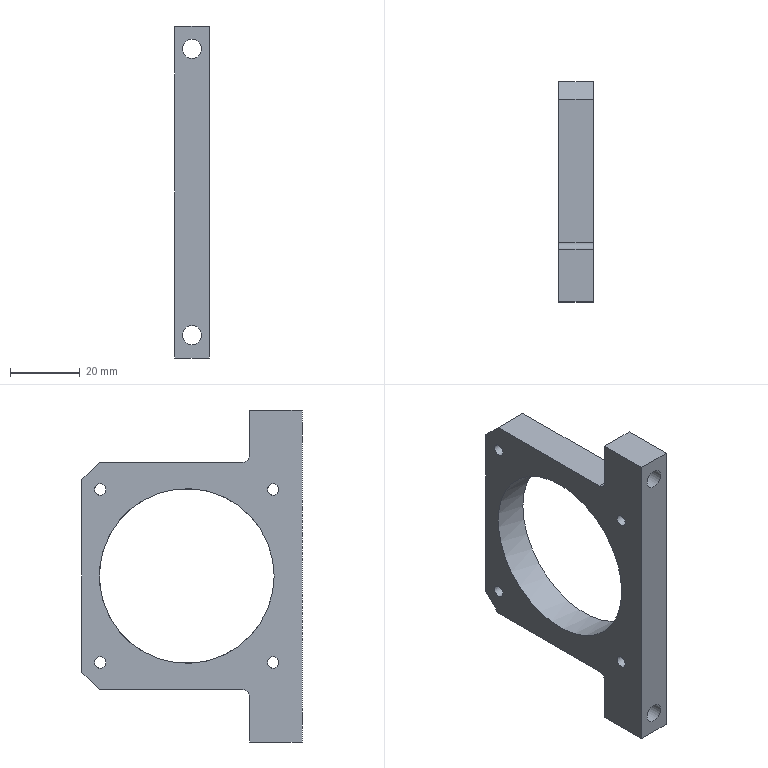Part | NX | 1 solid | 21 faces | box 10 x 63 x 95 mm | volume 24527 mm3 | plane 12 | cylinder 9 | commonest cylinder face diameters 3.3 x4 4 x2 5.5 x2 50 x1
STEP:
#1=CARTESIAN_POINT('',(-10.,42.749,-23.099));
#2=VERTEX_POINT('',#1);
#3=CARTESIAN_POINT('',(-10.,42.749,-24.749));
#4=DIRECTION('',(-1.,0.,0.));
#5=DIRECTION('',(0.,0.,1.));
#6=AXIS2_PLACEMENT_3D('',#3,#4,#5);
#7=CIRCLE('',#6,1.65);
#8=EDGE_CURVE('',#2,#2,#7,.T.);
#9=ORIENTED_EDGE('',*,*,#8,.F.);
#10=EDGE_LOOP('',(#9));
#11=FACE_BOUND('',#10,.T.);
#12=CARTESIAN_POINT('',(-10.,42.749,26.399));
#13=VERTEX_POINT('',#12);
#14=CARTESIAN_POINT('',(-10.,42.749,24.749));
#15=DIRECTION('',(-1.,0.,0.));
#16=DIRECTION('',(0.,0.,1.));
#17=AXIS2_PLACEMENT_3D('',#14,#15,#16);
#18=CIRCLE('',#17,1.65);
#19=EDGE_CURVE('',#13,#13,#18,.T.);
#20=ORIENTED_EDGE('',*,*,#19,.F.);
#21=EDGE_LOOP('',(#20));
#22=FACE_BOUND('',#21,.T.);
#23=CARTESIAN_POINT('',(-10.,-6.749,26.399));
#24=VERTEX_POINT('',#23);
#25=CARTESIAN_POINT('',(-10.,-6.749,24.749));
#26=DIRECTION('',(-1.,0.,0.));
#27=DIRECTION('',(0.,0.,1.));
#28=AXIS2_PLACEMENT_3D('',#25,#26,#27);
#29=CIRCLE('',#28,1.65);
#30=EDGE_CURVE('',#24,#24,#29,.T.);
#31=ORIENTED_EDGE('',*,*,#30,.F.);
#32=EDGE_LOOP('',(#31));
#33=FACE_BOUND('',#32,.T.);
#34=CARTESIAN_POINT('',(-10.,-6.749,-23.099));
#35=VERTEX_POINT('',#34);
#36=CARTESIAN_POINT('',(-10.,-6.749,-24.749));
#37=DIRECTION('',(-1.,0.,0.));
#38=DIRECTION('',(0.,0.,1.));
#39=AXIS2_PLACEMENT_3D('',#36,#37,#38);
#40=CIRCLE('',#39,1.65);
#41=EDGE_CURVE('',#35,#35,#40,.T.);
#42=ORIENTED_EDGE('',*,*,#41,.F.);
#43=EDGE_LOOP('',(#42));
#44=FACE_BOUND('',#43,.T.);
#45=CARTESIAN_POINT('',(-10.,-7.,0.));
#46=VERTEX_POINT('',#45);
#47=CARTESIAN_POINT('',(-10.,18.,0.));
#48=DIRECTION('',(-1.,0.,0.));
#49=DIRECTION('',(0.,-1.,0.));
#50=AXIS2_PLACEMENT_3D('',#47,#48,#49);
#51=CIRCLE('',#50,25.);
#52=EDGE_CURVE('',#46,#46,#51,.T.);
#53=ORIENTED_EDGE('',*,*,#52,.F.);
#54=EDGE_LOOP('',(#53));
#55=FACE_BOUND('',#54,.T.);
#56=CARTESIAN_POINT('',(-10.,48.,27.5));
#57=VERTEX_POINT('',#56);
#58=CARTESIAN_POINT('',(-10.,48.,-27.5));
#59=VERTEX_POINT('',#58);
#60=CARTESIAN_POINT('',(-10.,48.,32.5));
#61=DIRECTION('',(0.,0.,-1.));
#62=VECTOR('',#61,1000.);
#63=LINE('',#60,#62);
#64=EDGE_CURVE('',#57,#59,#63,.T.);
#65=ORIENTED_EDGE('',*,*,#64,.T.);
#66=CARTESIAN_POINT('',(-10.,43.,-32.5));
#67=VERTEX_POINT('',#66);
#68=CARTESIAN_POINT('',(-10.,43.,-32.5));
#69=DIRECTION('',(0.,0.7071,0.7071));
#70=VECTOR('',#69,1000.);
#71=LINE('',#68,#70);
#72=EDGE_CURVE('',#59,#67,#71,.F.);
#73=ORIENTED_EDGE('',*,*,#72,.T.);
#74=CARTESIAN_POINT('',(-10.,2.,-32.5));
#75=VERTEX_POINT('',#74);
#76=CARTESIAN_POINT('',(-10.,48.,-32.5));
#77=DIRECTION('',(0.,-1.,0.));
#78=VECTOR('',#77,1000.);
#79=LINE('',#76,#78);
#80=EDGE_CURVE('',#67,#75,#79,.T.);
#81=ORIENTED_EDGE('',*,*,#80,.T.);
#82=CARTESIAN_POINT('',(-10.,0.,-34.5));
#83=VERTEX_POINT('',#82);
#84=CARTESIAN_POINT('',(-10.,2.,-34.5));
#85=DIRECTION('',(1.,0.,0.));
#86=DIRECTION('',(0.,1.,0.));
#87=AXIS2_PLACEMENT_3D('',#84,#85,#86);
#88=CIRCLE('',#87,2.);
#89=EDGE_CURVE('',#75,#83,#88,.T.);
#90=ORIENTED_EDGE('',*,*,#89,.T.);
#91=CARTESIAN_POINT('',(-10.,0.,-47.5));
#92=VERTEX_POINT('',#91);
#93=CARTESIAN_POINT('',(-10.,0.,-47.5));
#94=DIRECTION('',(0.,0.,-1.));
#95=VECTOR('',#94,1000.);
#96=LINE('',#93,#95);
#97=EDGE_CURVE('',#83,#92,#96,.T.);
#98=ORIENTED_EDGE('',*,*,#97,.T.);
#99=CARTESIAN_POINT('',(-10.,-15.,-47.5));
#100=VERTEX_POINT('',#99);
#101=CARTESIAN_POINT('',(-10.,-15.,-47.5));
#102=DIRECTION('',(0.,1.,0.));
#103=VECTOR('',#102,1000.);
#104=LINE('',#101,#103);
#105=EDGE_CURVE('',#100,#92,#104,.T.);
#106=ORIENTED_EDGE('',*,*,#105,.F.);
#107=CARTESIAN_POINT('',(-10.,-15.,47.5));
#108=VERTEX_POINT('',#107);
#109=CARTESIAN_POINT('',(-10.,-15.,-47.5));
#110=DIRECTION('',(0.,0.,-1.));
#111=VECTOR('',#110,1000.);
#112=LINE('',#109,#111);
#113=EDGE_CURVE('',#108,#100,#112,.T.);
#114=ORIENTED_EDGE('',*,*,#113,.F.);
#115=CARTESIAN_POINT('',(-10.,0.,47.5));
#116=VERTEX_POINT('',#115);
#117=CARTESIAN_POINT('',(-10.,-15.,47.5));
#118=DIRECTION('',(0.,1.,0.));
#119=VECTOR('',#118,1000.);
#120=LINE('',#117,#119);
#121=EDGE_CURVE('',#108,#116,#120,.T.);
#122=ORIENTED_EDGE('',*,*,#121,.T.);
#123=CARTESIAN_POINT('',(-10.,0.,34.5));
#124=VERTEX_POINT('',#123);
#125=CARTESIAN_POINT('',(-10.,0.,-47.5));
#126=DIRECTION('',(0.,0.,-1.));
#127=VECTOR('',#126,1000.);
#128=LINE('',#125,#127);
#129=EDGE_CURVE('',#116,#124,#128,.T.);
#130=ORIENTED_EDGE('',*,*,#129,.T.);
#131=CARTESIAN_POINT('',(-10.,2.,32.5));
#132=VERTEX_POINT('',#131);
#133=CARTESIAN_POINT('',(-10.,2.,34.5));
#134=DIRECTION('',(1.,0.,0.));
#135=DIRECTION('',(0.,1.,0.));
#136=AXIS2_PLACEMENT_3D('',#133,#134,#135);
#137=CIRCLE('',#136,2.);
#138=EDGE_CURVE('',#124,#132,#137,.T.);
#139=ORIENTED_EDGE('',*,*,#138,.T.);
#140=CARTESIAN_POINT('',(-10.,43.,32.5));
#141=VERTEX_POINT('',#140);
#142=CARTESIAN_POINT('',(-10.,48.,32.5));
#143=DIRECTION('',(0.,-1.,0.));
#144=VECTOR('',#143,1000.);
#145=LINE('',#142,#144);
#146=EDGE_CURVE('',#141,#132,#145,.T.);
#147=ORIENTED_EDGE('',*,*,#146,.F.);
#148=CARTESIAN_POINT('',(-10.,48.,27.5));
#149=DIRECTION('',(0.,0.7071,-0.7071));
#150=VECTOR('',#149,1000.);
#151=LINE('',#148,#150);
#152=EDGE_CURVE('',#141,#57,#151,.T.);
#153=ORIENTED_EDGE('',*,*,#152,.T.);
#154=EDGE_LOOP('',(#65,#73,#81,#90,#98,#106,#114,#122,#130,#139,#147,#153));
#155=FACE_BOUND('',#154,.T.);
#156=CARTESIAN_POINT('',(-10.,48.,32.5));
#157=DIRECTION('',(1.,0.,0.));
#158=DIRECTION('',(0.,1.,0.));
#159=AXIS2_PLACEMENT_3D('',#156,#157,#158);
#160=PLANE('',#159);
#161=ADVANCED_FACE('',(#11,#22,#33,#44,#55,#155),#160,.F.);
#162=CARTESIAN_POINT('',(0.,44.399,-24.749));
#163=VERTEX_POINT('',#162);
#164=CARTESIAN_POINT('',(0.,42.749,-24.749));
#165=DIRECTION('',(1.,0.,0.));
#166=DIRECTION('',(0.,1.,0.));
#167=AXIS2_PLACEMENT_3D('',#164,#165,#166);
#168=CIRCLE('',#167,1.65);
#169=EDGE_CURVE('',#163,#163,#168,.T.);
#170=ORIENTED_EDGE('',*,*,#169,.F.);
#171=EDGE_LOOP('',(#170));
#172=FACE_BOUND('',#171,.T.);
#173=CARTESIAN_POINT('',(0.,44.399,24.749));
#174=VERTEX_POINT('',#173);
#175=CARTESIAN_POINT('',(0.,42.749,24.749));
#176=DIRECTION('',(1.,0.,0.));
#177=DIRECTION('',(0.,1.,0.));
#178=AXIS2_PLACEMENT_3D('',#175,#176,#177);
#179=CIRCLE('',#178,1.65);
#180=EDGE_CURVE('',#174,#174,#179,.T.);
#181=ORIENTED_EDGE('',*,*,#180,.F.);
#182=EDGE_LOOP('',(#181));
#183=FACE_BOUND('',#182,.T.);
#184=CARTESIAN_POINT('',(0.,-5.099,24.749));
#185=VERTEX_POINT('',#184);
#186=CARTESIAN_POINT('',(0.,-6.749,24.749));
#187=DIRECTION('',(1.,0.,0.));
#188=DIRECTION('',(0.,1.,0.));
#189=AXIS2_PLACEMENT_3D('',#186,#187,#188);
#190=CIRCLE('',#189,1.65);
#191=EDGE_CURVE('',#185,#185,#190,.T.);
#192=ORIENTED_EDGE('',*,*,#191,.F.);
#193=EDGE_LOOP('',(#192));
#194=FACE_BOUND('',#193,.T.);
#195=CARTESIAN_POINT('',(0.,-5.099,-24.749));
#196=VERTEX_POINT('',#195);
#197=CARTESIAN_POINT('',(0.,-6.749,-24.749));
#198=DIRECTION('',(1.,0.,0.));
#199=DIRECTION('',(0.,1.,0.));
#200=AXIS2_PLACEMENT_3D('',#197,#198,#199);
#201=CIRCLE('',#200,1.65);
#202=EDGE_CURVE('',#196,#196,#201,.T.);
#203=ORIENTED_EDGE('',*,*,#202,.F.);
#204=EDGE_LOOP('',(#203));
#205=FACE_BOUND('',#204,.T.);
#206=CARTESIAN_POINT('',(0.,43.,0.));
#207=VERTEX_POINT('',#206);
#208=CARTESIAN_POINT('',(0.,18.,0.));
#209=DIRECTION('',(1.,0.,0.));
#210=DIRECTION('',(0.,1.,0.));
#211=AXIS2_PLACEMENT_3D('',#208,#209,#210);
#212=CIRCLE('',#211,25.);
#213=EDGE_CURVE('',#207,#207,#212,.T.);
#214=ORIENTED_EDGE('',*,*,#213,.F.);
#215=EDGE_LOOP('',(#214));
#216=FACE_BOUND('',#215,.T.);
#217=CARTESIAN_POINT('',(0.,43.,-32.5));
#218=VERTEX_POINT('',#217);
#219=CARTESIAN_POINT('',(0.,2.,-32.5));
#220=VERTEX_POINT('',#219);
#221=CARTESIAN_POINT('',(0.,48.,-32.5));
#222=DIRECTION('',(0.,-1.,0.));
#223=VECTOR('',#222,1000.);
#224=LINE('',#221,#223);
#225=EDGE_CURVE('',#218,#220,#224,.T.);
#226=ORIENTED_EDGE('',*,*,#225,.F.);
#227=CARTESIAN_POINT('',(0.,48.,-27.5));
#228=VERTEX_POINT('',#227);
#229=CARTESIAN_POINT('',(0.,78.,2.5));
#230=DIRECTION('',(0.,-0.7071,-0.7071));
#231=VECTOR('',#230,1000.);
#232=LINE('',#229,#231);
#233=EDGE_CURVE('',#218,#228,#232,.F.);
#234=ORIENTED_EDGE('',*,*,#233,.T.);
#235=CARTESIAN_POINT('',(0.,48.,27.5));
#236=VERTEX_POINT('',#235);
#237=CARTESIAN_POINT('',(0.,48.,32.5));
#238=DIRECTION('',(0.,0.,-1.));
#239=VECTOR('',#238,1000.);
#240=LINE('',#237,#239);
#241=EDGE_CURVE('',#236,#228,#240,.T.);
#242=ORIENTED_EDGE('',*,*,#241,.F.);
#243=CARTESIAN_POINT('',(0.,43.,32.5));
#244=VERTEX_POINT('',#243);
#245=CARTESIAN_POINT('',(0.,45.5,30.));
#246=DIRECTION('',(0.,-0.7071,0.7071));
#247=VECTOR('',#246,1000.);
#248=LINE('',#245,#247);
#249=EDGE_CURVE('',#236,#244,#248,.T.);
#250=ORIENTED_EDGE('',*,*,#249,.T.);
#251=CARTESIAN_POINT('',(0.,2.,32.5));
#252=VERTEX_POINT('',#251);
#253=CARTESIAN_POINT('',(0.,48.,32.5));
#254=DIRECTION('',(0.,-1.,0.));
#255=VECTOR('',#254,1000.);
#256=LINE('',#253,#255);
#257=EDGE_CURVE('',#244,#252,#256,.T.);
#258=ORIENTED_EDGE('',*,*,#257,.T.);
#259=CARTESIAN_POINT('',(0.,0.,34.5));
#260=VERTEX_POINT('',#259);
#261=CARTESIAN_POINT('',(0.,2.,34.5));
#262=DIRECTION('',(1.,0.,0.));
#263=DIRECTION('',(0.,1.,0.));
#264=AXIS2_PLACEMENT_3D('',#261,#262,#263);
#265=CIRCLE('',#264,2.);
#266=EDGE_CURVE('',#252,#260,#265,.F.);
#267=ORIENTED_EDGE('',*,*,#266,.T.);
#268=CARTESIAN_POINT('',(0.,0.,47.5));
#269=VERTEX_POINT('',#268);
#270=CARTESIAN_POINT('',(0.,0.,-47.5));
#271=DIRECTION('',(0.,0.,1.));
#272=VECTOR('',#271,1000.);
#273=LINE('',#270,#272);
#274=EDGE_CURVE('',#260,#269,#273,.T.);
#275=ORIENTED_EDGE('',*,*,#274,.T.);
#276=CARTESIAN_POINT('',(0.,-15.,47.5));
#277=VERTEX_POINT('',#276);
#278=CARTESIAN_POINT('',(0.,-15.,47.5));
#279=DIRECTION('',(0.,1.,0.));
#280=VECTOR('',#279,1000.);
#281=LINE('',#278,#280);
#282=EDGE_CURVE('',#277,#269,#281,.T.);
#283=ORIENTED_EDGE('',*,*,#282,.F.);
#284=CARTESIAN_POINT('',(0.,-15.,-47.5));
#285=VERTEX_POINT('',#284);
#286=CARTESIAN_POINT('',(0.,-15.,-47.5));
#287=DIRECTION('',(0.,0.,1.));
#288=VECTOR('',#287,1000.);
#289=LINE('',#286,#288);
#290=EDGE_CURVE('',#285,#277,#289,.T.);
#291=ORIENTED_EDGE('',*,*,#290,.F.);
#292=CARTESIAN_POINT('',(0.,0.,-47.5));
#293=VERTEX_POINT('',#292);
#294=CARTESIAN_POINT('',(0.,-15.,-47.5));
#295=DIRECTION('',(0.,1.,0.));
#296=VECTOR('',#295,1000.);
#297=LINE('',#294,#296);
#298=EDGE_CURVE('',#285,#293,#297,.T.);
#299=ORIENTED_EDGE('',*,*,#298,.T.);
#300=CARTESIAN_POINT('',(0.,0.,-34.5));
#301=VERTEX_POINT('',#300);
#302=CARTESIAN_POINT('',(0.,0.,-47.5));
#303=DIRECTION('',(0.,0.,1.));
#304=VECTOR('',#303,1000.);
#305=LINE('',#302,#304);
#306=EDGE_CURVE('',#293,#301,#305,.T.);
#307=ORIENTED_EDGE('',*,*,#306,.T.);
#308=CARTESIAN_POINT('',(0.,2.,-34.5));
#309=DIRECTION('',(1.,0.,0.));
#310=DIRECTION('',(0.,1.,0.));
#311=AXIS2_PLACEMENT_3D('',#308,#309,#310);
#312=CIRCLE('',#311,2.);
#313=EDGE_CURVE('',#301,#220,#312,.F.);
#314=ORIENTED_EDGE('',*,*,#313,.T.);
#315=EDGE_LOOP('',(#226,#234,#242,#250,#258,#267,#275,#283,#291,#299,#307,#314));
#316=FACE_BOUND('',#315,.T.);
#317=CARTESIAN_POINT('',(0.,48.,32.5));
#318=DIRECTION('',(1.,0.,0.));
#319=DIRECTION('',(0.,1.,0.));
#320=AXIS2_PLACEMENT_3D('',#317,#318,#319);
#321=PLANE('',#320);
#322=ADVANCED_FACE('',(#172,#183,#194,#205,#216,#316),#321,.T.);
#323=ORIENTED_EDGE('',*,*,#241,.T.);
#324=CARTESIAN_POINT('',(-10.,48.,-27.5));
#325=DIRECTION('',(-1.,0.,0.));
#326=VECTOR('',#325,1000.);
#327=LINE('',#324,#326);
#328=EDGE_CURVE('',#228,#59,#327,.T.);
#329=ORIENTED_EDGE('',*,*,#328,.T.);
#330=ORIENTED_EDGE('',*,*,#64,.F.);
#331=CARTESIAN_POINT('',(0.,48.,27.5));
#332=DIRECTION('',(1.,0.,0.));
#333=VECTOR('',#332,1000.);
#334=LINE('',#331,#333);
#335=EDGE_CURVE('',#57,#236,#334,.T.);
#336=ORIENTED_EDGE('',*,*,#335,.T.);
#337=EDGE_LOOP('',(#323,#329,#330,#336));
#338=FACE_BOUND('',#337,.T.);
#339=CARTESIAN_POINT('',(-10.,48.,32.5));
#340=DIRECTION('',(0.,1.,0.));
#341=DIRECTION('',(0.,0.,1.));
#342=AXIS2_PLACEMENT_3D('',#339,#340,#341);
#343=PLANE('',#342);
#344=ADVANCED_FACE('',(#338),#343,.T.);
#345=ORIENTED_EDGE('',*,*,#146,.T.);
#346=CARTESIAN_POINT('',(0.,2.,32.5));
#347=DIRECTION('',(-1.,0.,0.));
#348=VECTOR('',#347,1000.);
#349=LINE('',#346,#348);
#350=EDGE_CURVE('',#132,#252,#349,.F.);
#351=ORIENTED_EDGE('',*,*,#350,.T.);
#352=ORIENTED_EDGE('',*,*,#257,.F.);
#353=CARTESIAN_POINT('',(-10.,43.,32.5));
#354=DIRECTION('',(-1.,0.,0.));
#355=VECTOR('',#354,1000.);
#356=LINE('',#353,#355);
#357=EDGE_CURVE('',#244,#141,#356,.T.);
#358=ORIENTED_EDGE('',*,*,#357,.T.);
#359=EDGE_LOOP('',(#345,#351,#352,#358));
#360=FACE_BOUND('',#359,.T.);
#361=CARTESIAN_POINT('',(0.,0.,32.5));
#362=DIRECTION('',(0.,0.,-1.));
#363=DIRECTION('',(-1.,0.,0.));
#364=AXIS2_PLACEMENT_3D('',#361,#362,#363);
#365=PLANE('',#364);
#366=ADVANCED_FACE('',(#360),#365,.F.);
#367=ORIENTED_EDGE('',*,*,#225,.T.);
#368=CARTESIAN_POINT('',(-10.,2.,-32.5));
#369=DIRECTION('',(-1.,0.,0.));
#370=VECTOR('',#369,1000.);
#371=LINE('',#368,#370);
#372=EDGE_CURVE('',#220,#75,#371,.T.);
#373=ORIENTED_EDGE('',*,*,#372,.T.);
#374=ORIENTED_EDGE('',*,*,#80,.F.);
#375=CARTESIAN_POINT('',(0.,43.,-32.5));
#376=DIRECTION('',(1.,0.,0.));
#377=VECTOR('',#376,1000.);
#378=LINE('',#375,#377);
#379=EDGE_CURVE('',#67,#218,#378,.T.);
#380=ORIENTED_EDGE('',*,*,#379,.T.);
#381=EDGE_LOOP('',(#367,#373,#374,#380));
#382=FACE_BOUND('',#381,.T.);
#383=CARTESIAN_POINT('',(0.,0.,-32.5));
#384=DIRECTION('',(0.,0.,-1.));
#385=DIRECTION('',(-1.,0.,0.));
#386=AXIS2_PLACEMENT_3D('',#383,#384,#385);
#387=PLANE('',#386);
#388=ADVANCED_FACE('',(#382),#387,.T.);
#389=CARTESIAN_POINT('',(-5.,0.,-38.25));
#390=VERTEX_POINT('',#389);
#391=CARTESIAN_POINT('',(-5.,0.,-41.));
#392=DIRECTION('',(0.,1.,0.));
#393=DIRECTION('',(0.,0.,1.));
#394=AXIS2_PLACEMENT_3D('',#391,#392,#393);
#395=CIRCLE('',#394,2.75);
#396=EDGE_CURVE('',#390,#390,#395,.T.);
#397=ORIENTED_EDGE('',*,*,#396,.F.);
#398=EDGE_LOOP('',(#397));
#399=FACE_BOUND('',#398,.T.);
#400=ORIENTED_EDGE('',*,*,#97,.F.);
#401=CARTESIAN_POINT('',(0.,0.,-34.5));
#402=DIRECTION('',(-1.,0.,0.));
#403=VECTOR('',#402,1000.);
#404=LINE('',#401,#403);
#405=EDGE_CURVE('',#83,#301,#404,.F.);
#406=ORIENTED_EDGE('',*,*,#405,.T.);
#407=ORIENTED_EDGE('',*,*,#306,.F.);
#408=CARTESIAN_POINT('',(-10.,0.,-47.5));
#409=DIRECTION('',(1.,0.,0.));
#410=VECTOR('',#409,1000.);
#411=LINE('',#408,#410);
#412=EDGE_CURVE('',#92,#293,#411,.T.);
#413=ORIENTED_EDGE('',*,*,#412,.F.);
#414=EDGE_LOOP('',(#400,#406,#407,#413));
#415=FACE_BOUND('',#414,.T.);
#416=CARTESIAN_POINT('',(0.,0.,0.));
#417=DIRECTION('',(0.,1.,0.));
#418=DIRECTION('',(0.,0.,1.));
#419=AXIS2_PLACEMENT_3D('',#416,#417,#418);
#420=PLANE('',#419);
#421=ADVANCED_FACE('',(#399,#415),#420,.T.);
#422=CARTESIAN_POINT('',(-10.,0.,47.5));
#423=DIRECTION('',(-1.,0.,0.));
#424=VECTOR('',#423,1000.);
#425=LINE('',#422,#424);
#426=EDGE_CURVE('',#269,#116,#425,.T.);
#427=ORIENTED_EDGE('',*,*,#426,.T.);
#428=ORIENTED_EDGE('',*,*,#121,.F.);
#429=CARTESIAN_POINT('',(-10.,-15.,47.5));
#430=DIRECTION('',(-1.,0.,0.));
#431=VECTOR('',#430,1000.);
#432=LINE('',#429,#431);
#433=EDGE_CURVE('',#277,#108,#432,.T.);
#434=ORIENTED_EDGE('',*,*,#433,.F.);
#435=ORIENTED_EDGE('',*,*,#282,.T.);
#436=EDGE_LOOP('',(#427,#428,#434,#435));
#437=FACE_BOUND('',#436,.T.);
#438=CARTESIAN_POINT('',(-10.,-15.,47.5));
#439=DIRECTION('',(0.,0.,-1.));
#440=DIRECTION('',(-1.,0.,0.));
#441=AXIS2_PLACEMENT_3D('',#438,#439,#440);
#442=PLANE('',#441);
#443=ADVANCED_FACE('',(#437),#442,.F.);
#444=ORIENTED_EDGE('',*,*,#412,.T.);
#445=ORIENTED_EDGE('',*,*,#298,.F.);
#446=CARTESIAN_POINT('',(-10.,-15.,-47.5));
#447=DIRECTION('',(1.,0.,0.));
#448=VECTOR('',#447,1000.);
#449=LINE('',#446,#448);
#450=EDGE_CURVE('',#100,#285,#449,.T.);
#451=ORIENTED_EDGE('',*,*,#450,.F.);
#452=ORIENTED_EDGE('',*,*,#105,.T.);
#453=EDGE_LOOP('',(#444,#445,#451,#452));
#454=FACE_BOUND('',#453,.T.);
#455=CARTESIAN_POINT('',(-10.,-15.,-47.5));
#456=DIRECTION('',(0.,0.,1.));
#457=DIRECTION('',(1.,0.,0.));
#458=AXIS2_PLACEMENT_3D('',#455,#456,#457);
#459=PLANE('',#458);
#460=ADVANCED_FACE('',(#454),#459,.F.);
#461=CARTESIAN_POINT('',(-5.,-15.,43.75));
#462=VERTEX_POINT('',#461);
#463=CARTESIAN_POINT('',(-5.,-15.,41.));
#464=DIRECTION('',(0.,1.,0.));
#465=DIRECTION('',(0.,0.,1.));
#466=AXIS2_PLACEMENT_3D('',#463,#464,#465);
#467=CIRCLE('',#466,2.75);
#468=EDGE_CURVE('',#462,#462,#467,.T.);
#469=ORIENTED_EDGE('',*,*,#468,.T.);
#470=EDGE_LOOP('',(#469));
#471=FACE_BOUND('',#470,.T.);
#472=CARTESIAN_POINT('',(-5.,-15.,-38.25));
#473=VERTEX_POINT('',#472);
#474=CARTESIAN_POINT('',(-5.,-15.,-41.));
#475=DIRECTION('',(0.,1.,0.));
#476=DIRECTION('',(0.,0.,1.));
#477=AXIS2_PLACEMENT_3D('',#474,#475,#476);
#478=CIRCLE('',#477,2.75);
#479=EDGE_CURVE('',#473,#473,#478,.T.);
#480=ORIENTED_EDGE('',*,*,#479,.T.);
#481=EDGE_LOOP('',(#480));
#482=FACE_BOUND('',#481,.T.);
#483=ORIENTED_EDGE('',*,*,#290,.T.);
#484=ORIENTED_EDGE('',*,*,#433,.T.);
#485=ORIENTED_EDGE('',*,*,#113,.T.);
#486=ORIENTED_EDGE('',*,*,#450,.T.);
#487=EDGE_LOOP('',(#483,#484,#485,#486));
#488=FACE_BOUND('',#487,.T.);
#489=CARTESIAN_POINT('',(0.,-15.,0.));
#490=DIRECTION('',(0.,1.,0.));
#491=DIRECTION('',(0.,0.,1.));
#492=AXIS2_PLACEMENT_3D('',#489,#490,#491);
#493=PLANE('',#492);
#494=ADVANCED_FACE('',(#471,#482,#488),#493,.F.);
#495=CARTESIAN_POINT('',(-5.,0.,43.75));
#496=VERTEX_POINT('',#495);
#497=CARTESIAN_POINT('',(-5.,0.,41.));
#498=DIRECTION('',(0.,1.,0.));
#499=DIRECTION('',(0.,0.,1.));
#500=AXIS2_PLACEMENT_3D('',#497,#498,#499);
#501=CIRCLE('',#500,2.75);
#502=EDGE_CURVE('',#496,#496,#501,.T.);
#503=ORIENTED_EDGE('',*,*,#502,.F.);
#504=EDGE_LOOP('',(#503));
#505=FACE_BOUND('',#504,.T.);
#506=ORIENTED_EDGE('',*,*,#274,.F.);
#507=CARTESIAN_POINT('',(0.,0.,34.5));
#508=DIRECTION('',(-1.,0.,0.));
#509=VECTOR('',#508,1000.);
#510=LINE('',#507,#509);
#511=EDGE_CURVE('',#260,#124,#510,.T.);
#512=ORIENTED_EDGE('',*,*,#511,.T.);
#513=ORIENTED_EDGE('',*,*,#129,.F.);
#514=ORIENTED_EDGE('',*,*,#426,.F.);
#515=EDGE_LOOP('',(#506,#512,#513,#514));
#516=FACE_BOUND('',#515,.T.);
#517=CARTESIAN_POINT('',(0.,0.,0.));
#518=DIRECTION('',(0.,1.,0.));
#519=DIRECTION('',(0.,0.,1.));
#520=AXIS2_PLACEMENT_3D('',#517,#518,#519);
#521=PLANE('',#520);
#522=ADVANCED_FACE('',(#505,#516),#521,.T.);
#523=ORIENTED_EDGE('',*,*,#213,.T.);
#524=EDGE_LOOP('',(#523));
#525=FACE_BOUND('',#524,.T.);
#526=ORIENTED_EDGE('',*,*,#52,.T.);
#527=EDGE_LOOP('',(#526));
#528=FACE_BOUND('',#527,.T.);
#529=CARTESIAN_POINT('',(0.00005,18.,0.));
#530=DIRECTION('',(-1.,0.,0.));
#531=DIRECTION('',(0.,-1.,0.));
#532=AXIS2_PLACEMENT_3D('',#529,#530,#531);
#533=CYLINDRICAL_SURFACE('',#532,25.);
#534=ADVANCED_FACE('',(#525,#528),#533,.F.);
#535=ORIENTED_EDGE('',*,*,#202,.T.);
#536=EDGE_LOOP('',(#535));
#537=FACE_BOUND('',#536,.T.);
#538=ORIENTED_EDGE('',*,*,#41,.T.);
#539=EDGE_LOOP('',(#538));
#540=FACE_BOUND('',#539,.T.);
#541=CARTESIAN_POINT('',(-10.,-6.749,-24.749));
#542=DIRECTION('',(-1.,0.,0.));
#543=DIRECTION('',(0.,0.,1.));
#544=AXIS2_PLACEMENT_3D('',#541,#542,#543);
#545=CYLINDRICAL_SURFACE('',#544,1.65);
#546=ADVANCED_FACE('',(#537,#540),#545,.F.);
#547=ORIENTED_EDGE('',*,*,#191,.T.);
#548=EDGE_LOOP('',(#547));
#549=FACE_BOUND('',#548,.T.);
#550=ORIENTED_EDGE('',*,*,#30,.T.);
#551=EDGE_LOOP('',(#550));
#552=FACE_BOUND('',#551,.T.);
#553=CARTESIAN_POINT('',(-10.,-6.749,24.749));
#554=DIRECTION('',(-1.,0.,0.));
#555=DIRECTION('',(0.,0.,1.));
#556=AXIS2_PLACEMENT_3D('',#553,#554,#555);
#557=CYLINDRICAL_SURFACE('',#556,1.65);
#558=ADVANCED_FACE('',(#549,#552),#557,.F.);
#559=ORIENTED_EDGE('',*,*,#180,.T.);
#560=EDGE_LOOP('',(#559));
#561=FACE_BOUND('',#560,.T.);
#562=ORIENTED_EDGE('',*,*,#19,.T.);
#563=EDGE_LOOP('',(#562));
#564=FACE_BOUND('',#563,.T.);
#565=CARTESIAN_POINT('',(-10.,42.749,24.749));
#566=DIRECTION('',(-1.,0.,0.));
#567=DIRECTION('',(0.,0.,1.));
#568=AXIS2_PLACEMENT_3D('',#565,#566,#567);
#569=CYLINDRICAL_SURFACE('',#568,1.65);
#570=ADVANCED_FACE('',(#561,#564),#569,.F.);
#571=ORIENTED_EDGE('',*,*,#169,.T.);
#572=EDGE_LOOP('',(#571));
#573=FACE_BOUND('',#572,.T.);
#574=ORIENTED_EDGE('',*,*,#8,.T.);
#575=EDGE_LOOP('',(#574));
#576=FACE_BOUND('',#575,.T.);
#577=CARTESIAN_POINT('',(-10.,42.749,-24.749));
#578=DIRECTION('',(-1.,0.,0.));
#579=DIRECTION('',(0.,0.,1.));
#580=AXIS2_PLACEMENT_3D('',#577,#578,#579);
#581=CYLINDRICAL_SURFACE('',#580,1.65);
#582=ADVANCED_FACE('',(#573,#576),#581,.F.);
#583=ORIENTED_EDGE('',*,*,#72,.F.);
#584=ORIENTED_EDGE('',*,*,#328,.F.);
#585=ORIENTED_EDGE('',*,*,#233,.F.);
#586=ORIENTED_EDGE('',*,*,#379,.F.);
#587=EDGE_LOOP('',(#583,#584,#585,#586));
#588=FACE_BOUND('',#587,.T.);
#589=CARTESIAN_POINT('',(0.,43.,-32.5));
#590=DIRECTION('',(0.,-0.7071,0.7071));
#591=DIRECTION('',(1.,0.,0.));
#592=AXIS2_PLACEMENT_3D('',#589,#590,#591);
#593=PLANE('',#592);
#594=ADVANCED_FACE('',(#588),#593,.F.);
#595=ORIENTED_EDGE('',*,*,#152,.F.);
#596=ORIENTED_EDGE('',*,*,#357,.F.);
#597=ORIENTED_EDGE('',*,*,#249,.F.);
#598=ORIENTED_EDGE('',*,*,#335,.F.);
#599=EDGE_LOOP('',(#595,#596,#597,#598));
#600=FACE_BOUND('',#599,.T.);
#601=CARTESIAN_POINT('',(-10.,48.,27.5));
#602=DIRECTION('',(0.,0.7071,0.7071));
#603=DIRECTION('',(-1.,0.,0.));
#604=AXIS2_PLACEMENT_3D('',#601,#602,#603);
#605=PLANE('',#604);
#606=ADVANCED_FACE('',(#600),#605,.T.);
#607=ORIENTED_EDGE('',*,*,#479,.F.);
#608=EDGE_LOOP('',(#607));
#609=FACE_BOUND('',#608,.T.);
#610=ORIENTED_EDGE('',*,*,#396,.T.);
#611=EDGE_LOOP('',(#610));
#612=FACE_BOUND('',#611,.T.);
#613=CARTESIAN_POINT('',(-5.,-15.,-41.));
#614=DIRECTION('',(0.,1.,0.));
#615=DIRECTION('',(0.,0.,1.));
#616=AXIS2_PLACEMENT_3D('',#613,#614,#615);
#617=CYLINDRICAL_SURFACE('',#616,2.75);
#618=ADVANCED_FACE('',(#609,#612),#617,.F.);
#619=ORIENTED_EDGE('',*,*,#468,.F.);
#620=EDGE_LOOP('',(#619));
#621=FACE_BOUND('',#620,.T.);
#622=ORIENTED_EDGE('',*,*,#502,.T.);
#623=EDGE_LOOP('',(#622));
#624=FACE_BOUND('',#623,.T.);
#625=CARTESIAN_POINT('',(-5.,-15.,41.));
#626=DIRECTION('',(0.,1.,0.));
#627=DIRECTION('',(0.,0.,1.));
#628=AXIS2_PLACEMENT_3D('',#625,#626,#627);
#629=CYLINDRICAL_SURFACE('',#628,2.75);
#630=ADVANCED_FACE('',(#621,#624),#629,.F.);
#631=ORIENTED_EDGE('',*,*,#313,.F.);
#632=ORIENTED_EDGE('',*,*,#405,.F.);
#633=ORIENTED_EDGE('',*,*,#89,.F.);
#634=ORIENTED_EDGE('',*,*,#372,.F.);
#635=EDGE_LOOP('',(#631,#632,#633,#634));
#636=FACE_BOUND('',#635,.T.);
#637=CARTESIAN_POINT('',(0.,2.,-34.5));
#638=DIRECTION('',(1.,0.,0.));
#639=DIRECTION('',(0.,0.,-1.));
#640=AXIS2_PLACEMENT_3D('',#637,#638,#639);
#641=CYLINDRICAL_SURFACE('',#640,2.);
#642=ADVANCED_FACE('',(#636),#641,.F.);
#643=ORIENTED_EDGE('',*,*,#266,.F.);
#644=ORIENTED_EDGE('',*,*,#350,.F.);
#645=ORIENTED_EDGE('',*,*,#138,.F.);
#646=ORIENTED_EDGE('',*,*,#511,.F.);
#647=EDGE_LOOP('',(#643,#644,#645,#646));
#648=FACE_BOUND('',#647,.T.);
#649=CARTESIAN_POINT('',(0.,2.,34.5));
#650=DIRECTION('',(-1.,0.,0.));
#651=DIRECTION('',(0.,0.,1.));
#652=AXIS2_PLACEMENT_3D('',#649,#650,#651);
#653=CYLINDRICAL_SURFACE('',#652,2.);
#654=ADVANCED_FACE('',(#648),#653,.F.);
#655=CLOSED_SHELL('',(#161,#322,#344,#366,#388,#421,#443,#460,#494,#522,#534,#546,#558,#570,#582,#594,#606,#618,#630,#642,#654));
#656=MANIFOLD_SOLID_BREP('',#655);
#657=(LENGTH_UNIT()NAMED_UNIT(*)SI_UNIT(.MILLI.,.METRE.));
#658=UNCERTAINTY_MEASURE_WITH_UNIT(LENGTH_MEASURE(0.00001),#657,'','');
#659=(NAMED_UNIT(*)PLANE_ANGLE_UNIT()SI_UNIT($,.RADIAN.));
#660=(NAMED_UNIT(*)SI_UNIT($,.STERADIAN.)SOLID_ANGLE_UNIT());
#661=(GEOMETRIC_REPRESENTATION_CONTEXT(3)GLOBAL_UNCERTAINTY_ASSIGNED_CONTEXT((#658))GLOBAL_UNIT_ASSIGNED_CONTEXT((#657,#659,#660))REPRESENTATION_CONTEXT('',''));
#662=ADVANCED_BREP_SHAPE_REPRESENTATION('',(#656),#661);